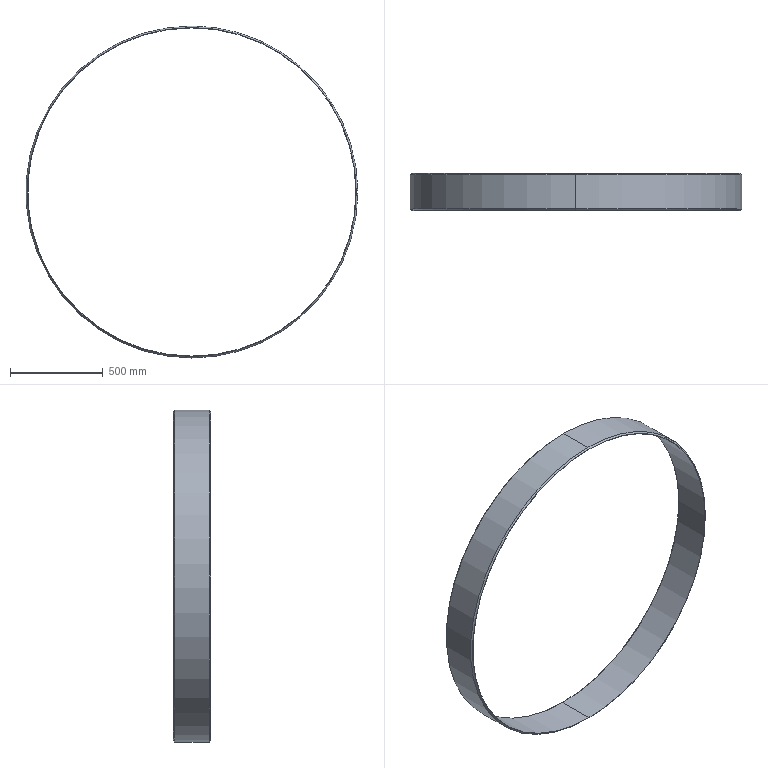Part | SolidWorks | features Chamfer 2, FlatPattern 1, SMBaseFlange 1, SheetMetal 1 | 1 solid | 16 faces | box 1790 x 200 x 1790 mm | volume 10805865 mm3 | cone 6 | cylinder 6 | plane 4 | commonest cylinder face diameters 1770 x3 1790 x3
STEP:
#1=CARTESIAN_POINT('',(0.,200.,887.));
#2=VERTEX_POINT('',#1);
#3=CARTESIAN_POINT('',(886.998,200.,2.097));
#4=VERTEX_POINT('',#3);
#5=CARTESIAN_POINT('',(0.,200.,0.));
#6=DIRECTION('',(0.,1.,0.));
#7=DIRECTION('',(0.,0.,1.));
#8=AXIS2_PLACEMENT_3D('',#5,#6,#7);
#9=CIRCLE('',#8,887.);
#10=EDGE_CURVE('',#2,#4,#9,.T.);
#11=ORIENTED_EDGE('',*,*,#10,.F.);
#12=CARTESIAN_POINT('',(0.,192.,895.));
#13=VERTEX_POINT('',#12);
#14=CARTESIAN_POINT('',(0.,200.,887.));
#15=DIRECTION('',(0.,-0.7071,0.7071));
#16=VECTOR('',#15,1000.);
#17=LINE('',#14,#16);
#18=EDGE_CURVE('',#2,#13,#17,.T.);
#19=ORIENTED_EDGE('',*,*,#18,.T.);
#20=CARTESIAN_POINT('',(894.944,192.,10.045));
#21=VERTEX_POINT('',#20);
#22=CARTESIAN_POINT('',(0.,192.,0.));
#23=DIRECTION('',(0.,-1.,0.));
#24=DIRECTION('',(0.,0.,1.));
#25=AXIS2_PLACEMENT_3D('',#22,#23,#24);
#26=CIRCLE('',#25,895.);
#27=EDGE_CURVE('',#21,#13,#26,.T.);
#28=ORIENTED_EDGE('',*,*,#27,.F.);
#29=CARTESIAN_POINT('',(894.944,192.,10.045));
#30=CARTESIAN_POINT('',(892.299,194.674,7.399));
#31=CARTESIAN_POINT('',(889.65,197.341,4.75));
#32=CARTESIAN_POINT('',(886.998,200.,2.097));
#33=B_SPLINE_CURVE_WITH_KNOTS('',3,(#29,#30,#31,#32),.UNSPECIFIED.,.F.,.F.,(4,4),(0.,0.0138),.UNSPECIFIED.);
#34=EDGE_CURVE('',#21,#4,#33,.T.);
#35=ORIENTED_EDGE('',*,*,#34,.T.);
#36=EDGE_LOOP('',(#11,#19,#28,#35));
#37=FACE_OUTER_BOUND('',#36,.T.);
#38=CARTESIAN_POINT('',(0.,200.,0.));
#39=DIRECTION('',(0.,-1.,0.));
#40=DIRECTION('',(0.,0.,-1.));
#41=AXIS2_PLACEMENT_3D('',#38,#39,#40);
#42=CONICAL_SURFACE('',#41,887.,0.7854);
#43=ADVANCED_FACE('',(#37),#42,.T.);
#44=ORIENTED_EDGE('',*,*,#18,.F.);
#45=CARTESIAN_POINT('',(0.,200.,-887.));
#46=VERTEX_POINT('',#45);
#47=CARTESIAN_POINT('',(0.,200.,0.));
#48=DIRECTION('',(0.,1.,0.));
#49=DIRECTION('',(0.,0.,1.));
#50=AXIS2_PLACEMENT_3D('',#47,#48,#49);
#51=CIRCLE('',#50,887.);
#52=EDGE_CURVE('',#46,#2,#51,.T.);
#53=ORIENTED_EDGE('',*,*,#52,.F.);
#54=CARTESIAN_POINT('',(0.,192.,-895.));
#55=VERTEX_POINT('',#54);
#56=CARTESIAN_POINT('',(0.,200.,-887.));
#57=DIRECTION('',(0.,-0.7071,-0.7071));
#58=VECTOR('',#57,1000.);
#59=LINE('',#56,#58);
#60=EDGE_CURVE('',#46,#55,#59,.T.);
#61=ORIENTED_EDGE('',*,*,#60,.T.);
#62=CARTESIAN_POINT('',(0.,192.,0.));
#63=DIRECTION('',(0.,-1.,0.));
#64=DIRECTION('',(0.,0.,1.));
#65=AXIS2_PLACEMENT_3D('',#62,#63,#64);
#66=CIRCLE('',#65,895.);
#67=EDGE_CURVE('',#13,#55,#66,.T.);
#68=ORIENTED_EDGE('',*,*,#67,.F.);
#69=EDGE_LOOP('',(#44,#53,#61,#68));
#70=FACE_OUTER_BOUND('',#69,.T.);
#71=CARTESIAN_POINT('',(0.,200.,0.));
#72=DIRECTION('',(0.,-1.,0.));
#73=DIRECTION('',(0.,0.,-1.));
#74=AXIS2_PLACEMENT_3D('',#71,#72,#73);
#75=CONICAL_SURFACE('',#74,887.,0.7854);
#76=ADVANCED_FACE('',(#70),#75,.T.);
#77=CARTESIAN_POINT('',(0.,0.,-887.));
#78=VERTEX_POINT('',#77);
#79=CARTESIAN_POINT('',(886.998,0.,-2.097));
#80=VERTEX_POINT('',#79);
#81=CARTESIAN_POINT('',(0.,0.,0.));
#82=DIRECTION('',(0.,-1.,0.));
#83=DIRECTION('',(0.,0.,1.));
#84=AXIS2_PLACEMENT_3D('',#81,#82,#83);
#85=CIRCLE('',#84,887.);
#86=EDGE_CURVE('',#78,#80,#85,.T.);
#87=ORIENTED_EDGE('',*,*,#86,.F.);
#88=CARTESIAN_POINT('',(0.,8.,-895.));
#89=VERTEX_POINT('',#88);
#90=CARTESIAN_POINT('',(0.,8.,-895.));
#91=DIRECTION('',(0.,0.7071,-0.7071));
#92=VECTOR('',#91,1000.);
#93=LINE('',#90,#92);
#94=EDGE_CURVE('',#78,#89,#93,.T.);
#95=ORIENTED_EDGE('',*,*,#94,.T.);
#96=CARTESIAN_POINT('',(894.944,8.,-10.045));
#97=VERTEX_POINT('',#96);
#98=CARTESIAN_POINT('',(0.,8.,0.));
#99=DIRECTION('',(0.,1.,0.));
#100=DIRECTION('',(0.,0.,1.));
#101=AXIS2_PLACEMENT_3D('',#98,#99,#100);
#102=CIRCLE('',#101,895.);
#103=EDGE_CURVE('',#97,#89,#102,.T.);
#104=ORIENTED_EDGE('',*,*,#103,.F.);
#105=CARTESIAN_POINT('',(894.944,8.,-10.045));
#106=CARTESIAN_POINT('',(892.299,5.326,-7.399));
#107=CARTESIAN_POINT('',(889.65,2.659,-4.75));
#108=CARTESIAN_POINT('',(886.998,0.,-2.097));
#109=B_SPLINE_CURVE_WITH_KNOTS('',3,(#105,#106,#107,#108),.UNSPECIFIED.,.F.,.F.,(4,4),(0.,0.0138),.UNSPECIFIED.);
#110=EDGE_CURVE('',#97,#80,#109,.T.);
#111=ORIENTED_EDGE('',*,*,#110,.T.);
#112=EDGE_LOOP('',(#87,#95,#104,#111));
#113=FACE_OUTER_BOUND('',#112,.T.);
#114=CARTESIAN_POINT('',(0.,8.,0.));
#115=DIRECTION('',(0.,1.,0.));
#116=DIRECTION('',(0.,0.,1.));
#117=AXIS2_PLACEMENT_3D('',#114,#115,#116);
#118=CONICAL_SURFACE('',#117,895.,0.7854);
#119=ADVANCED_FACE('',(#113),#118,.T.);
#120=ORIENTED_EDGE('',*,*,#94,.F.);
#121=CARTESIAN_POINT('',(0.,0.,887.));
#122=VERTEX_POINT('',#121);
#123=CARTESIAN_POINT('',(0.,0.,0.));
#124=DIRECTION('',(0.,-1.,0.));
#125=DIRECTION('',(0.,0.,1.));
#126=AXIS2_PLACEMENT_3D('',#123,#124,#125);
#127=CIRCLE('',#126,887.);
#128=EDGE_CURVE('',#122,#78,#127,.T.);
#129=ORIENTED_EDGE('',*,*,#128,.F.);
#130=CARTESIAN_POINT('',(0.,8.,895.));
#131=VERTEX_POINT('',#130);
#132=CARTESIAN_POINT('',(0.,8.,895.));
#133=DIRECTION('',(0.,0.7071,0.7071));
#134=VECTOR('',#133,1000.);
#135=LINE('',#132,#134);
#136=EDGE_CURVE('',#122,#131,#135,.T.);
#137=ORIENTED_EDGE('',*,*,#136,.T.);
#138=CARTESIAN_POINT('',(0.,8.,0.));
#139=DIRECTION('',(0.,1.,0.));
#140=DIRECTION('',(0.,0.,1.));
#141=AXIS2_PLACEMENT_3D('',#138,#139,#140);
#142=CIRCLE('',#141,895.);
#143=EDGE_CURVE('',#89,#131,#142,.T.);
#144=ORIENTED_EDGE('',*,*,#143,.F.);
#145=EDGE_LOOP('',(#120,#129,#137,#144));
#146=FACE_OUTER_BOUND('',#145,.T.);
#147=CARTESIAN_POINT('',(0.,8.,0.));
#148=DIRECTION('',(0.,1.,0.));
#149=DIRECTION('',(0.,0.,1.));
#150=AXIS2_PLACEMENT_3D('',#147,#148,#149);
#151=CONICAL_SURFACE('',#150,895.,0.7854);
#152=ADVANCED_FACE('',(#146),#151,.T.);
#153=CARTESIAN_POINT('',(0.,200.,-885.));
#154=VERTEX_POINT('',#153);
#155=CARTESIAN_POINT('',(0.,200.,885.));
#156=VERTEX_POINT('',#155);
#157=CARTESIAN_POINT('',(0.,200.,0.));
#158=DIRECTION('',(0.,1.,0.));
#159=DIRECTION('',(1.,0.,0.));
#160=AXIS2_PLACEMENT_3D('',#157,#158,#159);
#161=CIRCLE('',#160,885.);
#162=EDGE_CURVE('',#154,#156,#161,.T.);
#163=ORIENTED_EDGE('',*,*,#162,.T.);
#164=CARTESIAN_POINT('',(0.,0.,885.));
#165=VERTEX_POINT('',#164);
#166=CARTESIAN_POINT('',(0.,200.,885.));
#167=DIRECTION('',(0.,-1.,0.));
#168=VECTOR('',#167,1000.);
#169=LINE('',#166,#168);
#170=EDGE_CURVE('',#156,#165,#169,.T.);
#171=ORIENTED_EDGE('',*,*,#170,.T.);
#172=CARTESIAN_POINT('',(0.,0.,-885.));
#173=VERTEX_POINT('',#172);
#174=CARTESIAN_POINT('',(0.,0.,0.));
#175=DIRECTION('',(0.,1.,0.));
#176=DIRECTION('',(1.,0.,0.));
#177=AXIS2_PLACEMENT_3D('',#174,#175,#176);
#178=CIRCLE('',#177,885.);
#179=EDGE_CURVE('',#173,#165,#178,.T.);
#180=ORIENTED_EDGE('',*,*,#179,.F.);
#181=CARTESIAN_POINT('',(0.,200.,-885.));
#182=DIRECTION('',(0.,-1.,0.));
#183=VECTOR('',#182,1000.);
#184=LINE('',#181,#183);
#185=EDGE_CURVE('',#154,#173,#184,.T.);
#186=ORIENTED_EDGE('',*,*,#185,.F.);
#187=EDGE_LOOP('',(#163,#171,#180,#186));
#188=FACE_OUTER_BOUND('',#187,.T.);
#189=CARTESIAN_POINT('',(0.,200.,0.));
#190=DIRECTION('',(0.,-1.,0.));
#191=DIRECTION('',(0.,0.,-1.));
#192=AXIS2_PLACEMENT_3D('',#189,#190,#191);
#193=CYLINDRICAL_SURFACE('',#192,885.);
#194=ADVANCED_FACE('',(#188),#193,.F.);
#195=CARTESIAN_POINT('',(885.,200.,-0.09888));
#196=VERTEX_POINT('',#195);
#197=CARTESIAN_POINT('',(0.,200.,0.));
#198=DIRECTION('',(0.,1.,0.));
#199=DIRECTION('',(1.,0.,0.));
#200=AXIS2_PLACEMENT_3D('',#197,#198,#199);
#201=CIRCLE('',#200,885.);
#202=EDGE_CURVE('',#196,#154,#201,.T.);
#203=ORIENTED_EDGE('',*,*,#202,.T.);
#204=ORIENTED_EDGE('',*,*,#185,.T.);
#205=CARTESIAN_POINT('',(885.,0.,-0.09888));
#206=VERTEX_POINT('',#205);
#207=CARTESIAN_POINT('',(0.,0.,0.));
#208=DIRECTION('',(0.,1.,0.));
#209=DIRECTION('',(1.,0.,0.));
#210=AXIS2_PLACEMENT_3D('',#207,#208,#209);
#211=CIRCLE('',#210,885.);
#212=EDGE_CURVE('',#206,#173,#211,.T.);
#213=ORIENTED_EDGE('',*,*,#212,.F.);
#214=CARTESIAN_POINT('',(885.,200.,-0.09888));
#215=DIRECTION('',(0.,-1.,0.));
#216=VECTOR('',#215,1000.);
#217=LINE('',#214,#216);
#218=EDGE_CURVE('',#196,#206,#217,.T.);
#219=ORIENTED_EDGE('',*,*,#218,.F.);
#220=EDGE_LOOP('',(#203,#204,#213,#219));
#221=FACE_OUTER_BOUND('',#220,.T.);
#222=CARTESIAN_POINT('',(0.,200.,0.));
#223=DIRECTION('',(0.,-1.,0.));
#224=DIRECTION('',(0.,0.,-1.));
#225=AXIS2_PLACEMENT_3D('',#222,#223,#224);
#226=CYLINDRICAL_SURFACE('',#225,885.);
#227=ADVANCED_FACE('',(#221),#226,.F.);
#228=ORIENTED_EDGE('',*,*,#27,.T.);
#229=CARTESIAN_POINT('',(0.,200.,895.));
#230=DIRECTION('',(0.,-1.,0.));
#231=VECTOR('',#230,1000.);
#232=LINE('',#229,#231);
#233=EDGE_CURVE('',#13,#131,#232,.T.);
#234=ORIENTED_EDGE('',*,*,#233,.T.);
#235=CARTESIAN_POINT('',(894.944,8.,10.045));
#236=VERTEX_POINT('',#235);
#237=CARTESIAN_POINT('',(0.,8.,0.));
#238=DIRECTION('',(0.,1.,0.));
#239=DIRECTION('',(0.,0.,1.));
#240=AXIS2_PLACEMENT_3D('',#237,#238,#239);
#241=CIRCLE('',#240,895.);
#242=EDGE_CURVE('',#131,#236,#241,.T.);
#243=ORIENTED_EDGE('',*,*,#242,.T.);
#244=CARTESIAN_POINT('',(894.944,200.,10.045));
#245=DIRECTION('',(0.,1.,0.));
#246=VECTOR('',#245,1000.);
#247=LINE('',#244,#246);
#248=EDGE_CURVE('',#236,#21,#247,.T.);
#249=ORIENTED_EDGE('',*,*,#248,.T.);
#250=EDGE_LOOP('',(#228,#234,#243,#249));
#251=FACE_OUTER_BOUND('',#250,.T.);
#252=CARTESIAN_POINT('',(0.,200.,0.));
#253=DIRECTION('',(0.,-1.,0.));
#254=DIRECTION('',(0.,0.,-1.));
#255=AXIS2_PLACEMENT_3D('',#252,#253,#254);
#256=CYLINDRICAL_SURFACE('',#255,895.);
#257=ADVANCED_FACE('',(#251),#256,.T.);
#258=ORIENTED_EDGE('',*,*,#233,.F.);
#259=ORIENTED_EDGE('',*,*,#67,.T.);
#260=CARTESIAN_POINT('',(0.,200.,-895.));
#261=DIRECTION('',(0.,-1.,0.));
#262=VECTOR('',#261,1000.);
#263=LINE('',#260,#262);
#264=EDGE_CURVE('',#55,#89,#263,.T.);
#265=ORIENTED_EDGE('',*,*,#264,.T.);
#266=ORIENTED_EDGE('',*,*,#143,.T.);
#267=EDGE_LOOP('',(#258,#259,#265,#266));
#268=FACE_OUTER_BOUND('',#267,.T.);
#269=CARTESIAN_POINT('',(0.,200.,0.));
#270=DIRECTION('',(0.,-1.,0.));
#271=DIRECTION('',(0.,0.,-1.));
#272=AXIS2_PLACEMENT_3D('',#269,#270,#271);
#273=CYLINDRICAL_SURFACE('',#272,895.);
#274=ADVANCED_FACE('',(#268),#273,.T.);
#275=ORIENTED_EDGE('',*,*,#264,.F.);
#276=CARTESIAN_POINT('',(894.944,192.,-10.045));
#277=VERTEX_POINT('',#276);
#278=CARTESIAN_POINT('',(0.,192.,0.));
#279=DIRECTION('',(0.,-1.,0.));
#280=DIRECTION('',(0.,0.,1.));
#281=AXIS2_PLACEMENT_3D('',#278,#279,#280);
#282=CIRCLE('',#281,895.);
#283=EDGE_CURVE('',#55,#277,#282,.T.);
#284=ORIENTED_EDGE('',*,*,#283,.T.);
#285=CARTESIAN_POINT('',(894.944,200.,-10.045));
#286=DIRECTION('',(0.,-1.,0.));
#287=VECTOR('',#286,1000.);
#288=LINE('',#285,#287);
#289=EDGE_CURVE('',#277,#97,#288,.T.);
#290=ORIENTED_EDGE('',*,*,#289,.T.);
#291=ORIENTED_EDGE('',*,*,#103,.T.);
#292=EDGE_LOOP('',(#275,#284,#290,#291));
#293=FACE_OUTER_BOUND('',#292,.T.);
#294=CARTESIAN_POINT('',(0.,200.,0.));
#295=DIRECTION('',(0.,-1.,0.));
#296=DIRECTION('',(0.,0.,-1.));
#297=AXIS2_PLACEMENT_3D('',#294,#295,#296);
#298=CYLINDRICAL_SURFACE('',#297,895.);
#299=ADVANCED_FACE('',(#293),#298,.T.);
#300=ORIENTED_EDGE('',*,*,#170,.F.);
#301=CARTESIAN_POINT('',(885.,200.,0.09888));
#302=VERTEX_POINT('',#301);
#303=CARTESIAN_POINT('',(0.,200.,0.));
#304=DIRECTION('',(0.,1.,0.));
#305=DIRECTION('',(1.,0.,0.));
#306=AXIS2_PLACEMENT_3D('',#303,#304,#305);
#307=CIRCLE('',#306,885.);
#308=EDGE_CURVE('',#156,#302,#307,.T.);
#309=ORIENTED_EDGE('',*,*,#308,.T.);
#310=CARTESIAN_POINT('',(885.,0.,0.09888));
#311=VERTEX_POINT('',#310);
#312=CARTESIAN_POINT('',(885.,200.,0.09888));
#313=DIRECTION('',(0.,-1.,0.));
#314=VECTOR('',#313,1000.);
#315=LINE('',#312,#314);
#316=EDGE_CURVE('',#302,#311,#315,.T.);
#317=ORIENTED_EDGE('',*,*,#316,.T.);
#318=CARTESIAN_POINT('',(0.,0.,0.));
#319=DIRECTION('',(0.,1.,0.));
#320=DIRECTION('',(1.,0.,0.));
#321=AXIS2_PLACEMENT_3D('',#318,#319,#320);
#322=CIRCLE('',#321,885.);
#323=EDGE_CURVE('',#165,#311,#322,.T.);
#324=ORIENTED_EDGE('',*,*,#323,.F.);
#325=EDGE_LOOP('',(#300,#309,#317,#324));
#326=FACE_OUTER_BOUND('',#325,.T.);
#327=CARTESIAN_POINT('',(0.,200.,0.));
#328=DIRECTION('',(0.,-1.,0.));
#329=DIRECTION('',(0.,0.,-1.));
#330=AXIS2_PLACEMENT_3D('',#327,#328,#329);
#331=CYLINDRICAL_SURFACE('',#330,885.);
#332=ADVANCED_FACE('',(#326),#331,.F.);
#333=CARTESIAN_POINT('',(886.998,200.,-2.097));
#334=VERTEX_POINT('',#333);
#335=CARTESIAN_POINT('',(0.,200.,0.));
#336=DIRECTION('',(0.,1.,0.));
#337=DIRECTION('',(0.,0.,1.));
#338=AXIS2_PLACEMENT_3D('',#335,#336,#337);
#339=CIRCLE('',#338,887.);
#340=EDGE_CURVE('',#334,#46,#339,.T.);
#341=ORIENTED_EDGE('',*,*,#340,.T.);
#342=ORIENTED_EDGE('',*,*,#52,.T.);
#343=ORIENTED_EDGE('',*,*,#10,.T.);
#344=CARTESIAN_POINT('',(442.549,200.,-442.451));
#345=DIRECTION('',(-0.707,0.,-0.7072));
#346=VECTOR('',#345,1000.);
#347=LINE('',#344,#346);
#348=EDGE_CURVE('',#4,#302,#347,.T.);
#349=ORIENTED_EDGE('',*,*,#348,.T.);
#350=ORIENTED_EDGE('',*,*,#308,.F.);
#351=ORIENTED_EDGE('',*,*,#162,.F.);
#352=ORIENTED_EDGE('',*,*,#202,.F.);
#353=CARTESIAN_POINT('',(442.549,200.,442.451));
#354=DIRECTION('',(0.707,0.,-0.7072));
#355=VECTOR('',#354,1000.);
#356=LINE('',#353,#355);
#357=EDGE_CURVE('',#196,#334,#356,.T.);
#358=ORIENTED_EDGE('',*,*,#357,.T.);
#359=EDGE_LOOP('',(#341,#342,#343,#349,#350,#351,#352,#358));
#360=FACE_OUTER_BOUND('',#359,.T.);
#361=CARTESIAN_POINT('',(0.,200.,0.));
#362=DIRECTION('',(0.,1.,0.));
#363=DIRECTION('',(1.,0.,0.));
#364=AXIS2_PLACEMENT_3D('',#361,#362,#363);
#365=PLANE('',#364);
#366=ADVANCED_FACE('',(#360),#365,.T.);
#367=ORIENTED_EDGE('',*,*,#212,.T.);
#368=ORIENTED_EDGE('',*,*,#179,.T.);
#369=ORIENTED_EDGE('',*,*,#323,.T.);
#370=CARTESIAN_POINT('',(886.998,0.,2.097));
#371=VERTEX_POINT('',#370);
#372=CARTESIAN_POINT('',(885.,0.,0.09888));
#373=DIRECTION('',(0.707,0.,0.7072));
#374=VECTOR('',#373,1000.);
#375=LINE('',#372,#374);
#376=EDGE_CURVE('',#311,#371,#375,.T.);
#377=ORIENTED_EDGE('',*,*,#376,.T.);
#378=CARTESIAN_POINT('',(0.,0.,0.));
#379=DIRECTION('',(0.,-1.,0.));
#380=DIRECTION('',(0.,0.,1.));
#381=AXIS2_PLACEMENT_3D('',#378,#379,#380);
#382=CIRCLE('',#381,887.);
#383=EDGE_CURVE('',#371,#122,#382,.T.);
#384=ORIENTED_EDGE('',*,*,#383,.T.);
#385=ORIENTED_EDGE('',*,*,#128,.T.);
#386=ORIENTED_EDGE('',*,*,#86,.T.);
#387=CARTESIAN_POINT('',(894.944,0.,-10.045));
#388=DIRECTION('',(-0.707,0.,0.7072));
#389=VECTOR('',#388,1000.);
#390=LINE('',#387,#389);
#391=EDGE_CURVE('',#80,#206,#390,.T.);
#392=ORIENTED_EDGE('',*,*,#391,.T.);
#393=EDGE_LOOP('',(#367,#368,#369,#377,#384,#385,#386,#392));
#394=FACE_OUTER_BOUND('',#393,.T.);
#395=CARTESIAN_POINT('',(0.,0.,0.));
#396=DIRECTION('',(0.,1.,0.));
#397=DIRECTION('',(1.,0.,0.));
#398=AXIS2_PLACEMENT_3D('',#395,#396,#397);
#399=PLANE('',#398);
#400=ADVANCED_FACE('',(#394),#399,.F.);
#401=ORIENTED_EDGE('',*,*,#136,.F.);
#402=ORIENTED_EDGE('',*,*,#383,.F.);
#403=CARTESIAN_POINT('',(886.998,0.,2.097));
#404=CARTESIAN_POINT('',(889.65,2.659,4.75));
#405=CARTESIAN_POINT('',(892.299,5.326,7.399));
#406=CARTESIAN_POINT('',(894.944,8.,10.045));
#407=B_SPLINE_CURVE_WITH_KNOTS('',3,(#403,#404,#405,#406),.UNSPECIFIED.,.F.,.F.,(4,4),(0.,0.0138),.UNSPECIFIED.);
#408=EDGE_CURVE('',#371,#236,#407,.T.);
#409=ORIENTED_EDGE('',*,*,#408,.T.);
#410=ORIENTED_EDGE('',*,*,#242,.F.);
#411=EDGE_LOOP('',(#401,#402,#409,#410));
#412=FACE_OUTER_BOUND('',#411,.T.);
#413=CARTESIAN_POINT('',(0.,8.,0.));
#414=DIRECTION('',(0.,1.,0.));
#415=DIRECTION('',(0.,0.,1.));
#416=AXIS2_PLACEMENT_3D('',#413,#414,#415);
#417=CONICAL_SURFACE('',#416,895.,0.7854);
#418=ADVANCED_FACE('',(#412),#417,.T.);
#419=ORIENTED_EDGE('',*,*,#60,.F.);
#420=ORIENTED_EDGE('',*,*,#340,.F.);
#421=CARTESIAN_POINT('',(886.998,200.,-2.097));
#422=CARTESIAN_POINT('',(889.65,197.341,-4.75));
#423=CARTESIAN_POINT('',(892.299,194.674,-7.399));
#424=CARTESIAN_POINT('',(894.944,192.,-10.045));
#425=B_SPLINE_CURVE_WITH_KNOTS('',3,(#421,#422,#423,#424),.UNSPECIFIED.,.F.,.F.,(4,4),(0.,0.0138),.UNSPECIFIED.);
#426=EDGE_CURVE('',#334,#277,#425,.T.);
#427=ORIENTED_EDGE('',*,*,#426,.T.);
#428=ORIENTED_EDGE('',*,*,#283,.F.);
#429=EDGE_LOOP('',(#419,#420,#427,#428));
#430=FACE_OUTER_BOUND('',#429,.T.);
#431=CARTESIAN_POINT('',(0.,200.,0.));
#432=DIRECTION('',(0.,-1.,0.));
#433=DIRECTION('',(0.,0.,-1.));
#434=AXIS2_PLACEMENT_3D('',#431,#432,#433);
#435=CONICAL_SURFACE('',#434,887.,0.7854);
#436=ADVANCED_FACE('',(#430),#435,.T.);
#437=ORIENTED_EDGE('',*,*,#34,.F.);
#438=ORIENTED_EDGE('',*,*,#248,.F.);
#439=ORIENTED_EDGE('',*,*,#408,.F.);
#440=ORIENTED_EDGE('',*,*,#376,.F.);
#441=ORIENTED_EDGE('',*,*,#316,.F.);
#442=ORIENTED_EDGE('',*,*,#348,.F.);
#443=EDGE_LOOP('',(#437,#438,#439,#440,#441,#442));
#444=FACE_OUTER_BOUND('',#443,.T.);
#445=CARTESIAN_POINT('',(885.,200.,0.09888));
#446=DIRECTION('',(-0.7072,0.,0.707));
#447=DIRECTION('',(0.,-1.,0.));
#448=AXIS2_PLACEMENT_3D('',#445,#446,#447);
#449=PLANE('',#448);
#450=ADVANCED_FACE('',(#444),#449,.F.);
#451=ORIENTED_EDGE('',*,*,#357,.F.);
#452=ORIENTED_EDGE('',*,*,#218,.T.);
#453=ORIENTED_EDGE('',*,*,#391,.F.);
#454=ORIENTED_EDGE('',*,*,#110,.F.);
#455=ORIENTED_EDGE('',*,*,#289,.F.);
#456=ORIENTED_EDGE('',*,*,#426,.F.);
#457=EDGE_LOOP('',(#451,#452,#453,#454,#455,#456));
#458=FACE_OUTER_BOUND('',#457,.T.);
#459=CARTESIAN_POINT('',(894.944,200.,-10.045));
#460=DIRECTION('',(-0.7072,0.,-0.707));
#461=DIRECTION('',(0.,-1.,0.));
#462=AXIS2_PLACEMENT_3D('',#459,#460,#461);
#463=PLANE('',#462);
#464=ADVANCED_FACE('',(#458),#463,.F.);
#465=CLOSED_SHELL('',(#43,#76,#119,#152,#194,#227,#257,#274,#299,#332,#366,#400,#418,#436,#450,#464));
#466=MANIFOLD_SOLID_BREP('',#465);
#467=CARTESIAN_POINT('',(0.,0.,0.));
#468=DIRECTION('',(0.,0.,1.));
#469=DIRECTION('',(1.,0.,0.));
#470=AXIS2_PLACEMENT_3D('',#467,#468,#469);
#471=(LENGTH_UNIT()NAMED_UNIT(*)SI_UNIT(.MILLI.,.METRE.));
#472=UNCERTAINTY_MEASURE_WITH_UNIT(LENGTH_MEASURE(0.00001),#471,'','');
#473=(NAMED_UNIT(*)PLANE_ANGLE_UNIT()SI_UNIT($,.RADIAN.));
#474=(NAMED_UNIT(*)SI_UNIT($,.STERADIAN.)SOLID_ANGLE_UNIT());
#475=(GEOMETRIC_REPRESENTATION_CONTEXT(3)GLOBAL_UNCERTAINTY_ASSIGNED_CONTEXT((#472))GLOBAL_UNIT_ASSIGNED_CONTEXT((#471,#473,#474))REPRESENTATION_CONTEXT('',''));
#476=ADVANCED_BREP_SHAPE_REPRESENTATION('',(#466,#470),#475);